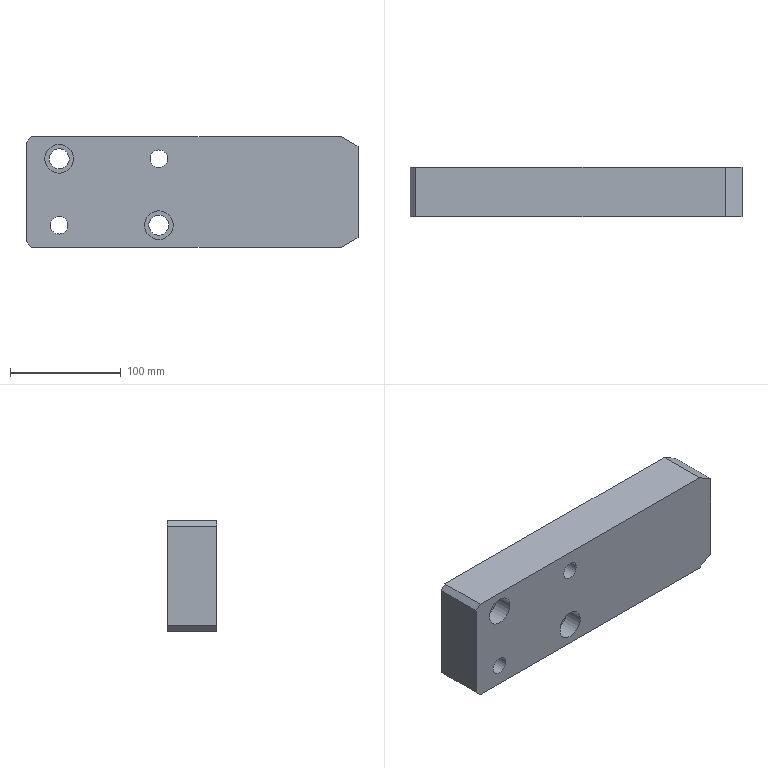Part | STEP file | solid 162 | 1 solid | 18 faces | box 300 x 45 x 100 mm | volume 1292632 mm3 | plane 12 | cylinder 6 | commonest cylinder face diameters 16 x2 18 x2 26 x2